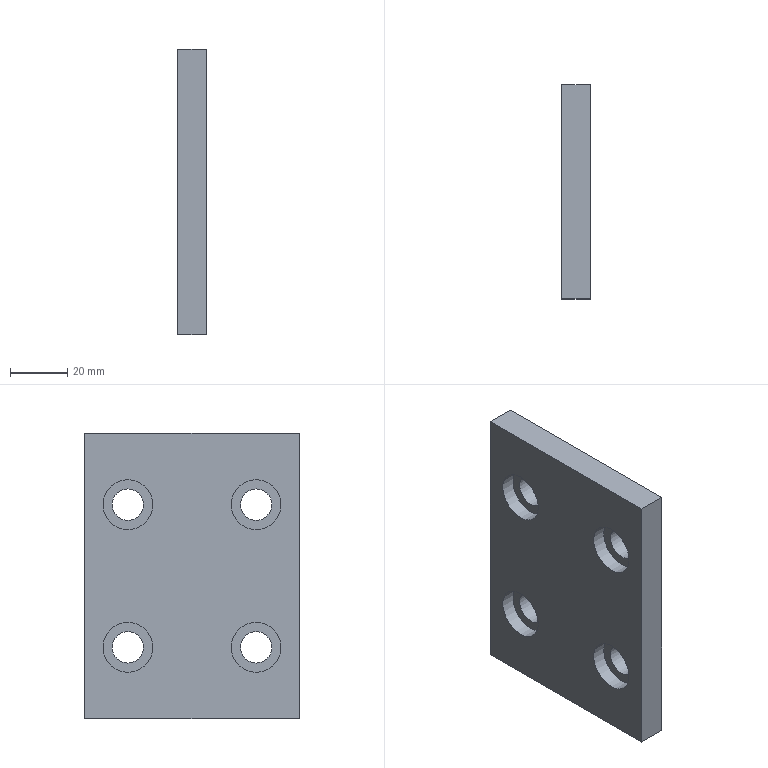Part | NX | features solid 2 | 1 solid | 18 faces | box 10 x 75 x 100 mm | volume 68289 mm3 | plane 10 | cylinder 8 | commonest cylinder face diameters 11 x4 17.5 x4
STEP:
#1=CARTESIAN_POINT('',(-885.,-217.5,218.75));
#2=VERTEX_POINT('',#1);
#3=CARTESIAN_POINT('',(-885.,-217.5,210.));
#4=DIRECTION('',(-1.,0.,0.));
#5=DIRECTION('',(0.,0.,1.));
#6=AXIS2_PLACEMENT_3D('',#3,#4,#5);
#7=CIRCLE('',#6,8.75);
#8=EDGE_CURVE('',#2,#2,#7,.T.);
#9=ORIENTED_EDGE('',*,*,#8,.T.);
#10=EDGE_LOOP('',(#9));
#11=FACE_BOUND('',#10,.T.);
#12=CARTESIAN_POINT('',(-885.,-217.5,204.5));
#13=VERTEX_POINT('',#12);
#14=CARTESIAN_POINT('',(-885.,-217.5,210.));
#15=DIRECTION('',(1.,0.,0.));
#16=DIRECTION('',(0.,0.,-1.));
#17=AXIS2_PLACEMENT_3D('',#14,#15,#16);
#18=CIRCLE('',#17,5.5);
#19=EDGE_CURVE('',#13,#13,#18,.F.);
#20=ORIENTED_EDGE('',*,*,#19,.F.);
#21=EDGE_LOOP('',(#20));
#22=FACE_BOUND('',#21,.T.);
#23=CARTESIAN_POINT('',(-885.,-217.5,210.));
#24=DIRECTION('',(1.,0.,0.));
#25=DIRECTION('',(0.,0.,-1.));
#26=AXIS2_PLACEMENT_3D('',#23,#24,#25);
#27=PLANE('',#26);
#28=ADVANCED_FACE('',(#11,#22),#27,.F.);
#29=CARTESIAN_POINT('',(-885.,-217.5,168.75));
#30=VERTEX_POINT('',#29);
#31=CARTESIAN_POINT('',(-885.,-217.5,160.));
#32=DIRECTION('',(-1.,0.,0.));
#33=DIRECTION('',(0.,0.,1.));
#34=AXIS2_PLACEMENT_3D('',#31,#32,#33);
#35=CIRCLE('',#34,8.75);
#36=EDGE_CURVE('',#30,#30,#35,.T.);
#37=ORIENTED_EDGE('',*,*,#36,.T.);
#38=EDGE_LOOP('',(#37));
#39=FACE_BOUND('',#38,.T.);
#40=CARTESIAN_POINT('',(-885.,-217.5,154.5));
#41=VERTEX_POINT('',#40);
#42=CARTESIAN_POINT('',(-885.,-217.5,160.));
#43=DIRECTION('',(1.,0.,0.));
#44=DIRECTION('',(0.,0.,-1.));
#45=AXIS2_PLACEMENT_3D('',#42,#43,#44);
#46=CIRCLE('',#45,5.5);
#47=EDGE_CURVE('',#41,#41,#46,.F.);
#48=ORIENTED_EDGE('',*,*,#47,.F.);
#49=EDGE_LOOP('',(#48));
#50=FACE_BOUND('',#49,.T.);
#51=CARTESIAN_POINT('',(-885.,-217.5,160.));
#52=DIRECTION('',(1.,0.,0.));
#53=DIRECTION('',(0.,0.,-1.));
#54=AXIS2_PLACEMENT_3D('',#51,#52,#53);
#55=PLANE('',#54);
#56=ADVANCED_FACE('',(#39,#50),#55,.F.);
#57=CARTESIAN_POINT('',(-890.,-217.5,218.75));
#58=VERTEX_POINT('',#57);
#59=CARTESIAN_POINT('',(-890.,-217.5,210.));
#60=DIRECTION('',(-1.,0.,0.));
#61=DIRECTION('',(0.,0.,1.));
#62=AXIS2_PLACEMENT_3D('',#59,#60,#61);
#63=CIRCLE('',#62,8.75);
#64=EDGE_CURVE('',#58,#58,#63,.F.);
#65=ORIENTED_EDGE('',*,*,#64,.F.);
#66=EDGE_LOOP('',(#65));
#67=FACE_BOUND('',#66,.T.);
#68=ORIENTED_EDGE('',*,*,#8,.F.);
#69=EDGE_LOOP('',(#68));
#70=FACE_BOUND('',#69,.T.);
#71=CARTESIAN_POINT('',(-885.,-217.5,210.));
#72=DIRECTION('',(-1.,0.,0.));
#73=DIRECTION('',(0.,0.,1.));
#74=AXIS2_PLACEMENT_3D('',#71,#72,#73);
#75=CYLINDRICAL_SURFACE('',#74,8.75);
#76=ADVANCED_FACE('',(#67,#70),#75,.F.);
#77=CARTESIAN_POINT('',(-890.,-217.5,168.75));
#78=VERTEX_POINT('',#77);
#79=CARTESIAN_POINT('',(-890.,-217.5,160.));
#80=DIRECTION('',(-1.,0.,0.));
#81=DIRECTION('',(0.,0.,1.));
#82=AXIS2_PLACEMENT_3D('',#79,#80,#81);
#83=CIRCLE('',#82,8.75);
#84=EDGE_CURVE('',#78,#78,#83,.F.);
#85=ORIENTED_EDGE('',*,*,#84,.F.);
#86=EDGE_LOOP('',(#85));
#87=FACE_BOUND('',#86,.T.);
#88=ORIENTED_EDGE('',*,*,#36,.F.);
#89=EDGE_LOOP('',(#88));
#90=FACE_BOUND('',#89,.T.);
#91=CARTESIAN_POINT('',(-885.,-217.5,160.));
#92=DIRECTION('',(-1.,0.,0.));
#93=DIRECTION('',(0.,0.,1.));
#94=AXIS2_PLACEMENT_3D('',#91,#92,#93);
#95=CYLINDRICAL_SURFACE('',#94,8.75);
#96=ADVANCED_FACE('',(#87,#90),#95,.F.);
#97=CARTESIAN_POINT('',(-890.,-202.5,135.));
#98=VERTEX_POINT('',#97);
#99=CARTESIAN_POINT('',(-890.,-202.5,235.));
#100=VERTEX_POINT('',#99);
#101=CARTESIAN_POINT('',(-890.,-202.5,135.));
#102=DIRECTION('',(0.,0.,1.));
#103=VECTOR('',#102,1000.);
#104=LINE('',#101,#103);
#105=EDGE_CURVE('',#98,#100,#104,.T.);
#106=ORIENTED_EDGE('',*,*,#105,.T.);
#107=CARTESIAN_POINT('',(-880.,-202.5,235.));
#108=VERTEX_POINT('',#107);
#109=CARTESIAN_POINT('',(-890.,-202.5,235.));
#110=DIRECTION('',(1.,0.,0.));
#111=VECTOR('',#110,1000.);
#112=LINE('',#109,#111);
#113=EDGE_CURVE('',#100,#108,#112,.T.);
#114=ORIENTED_EDGE('',*,*,#113,.T.);
#115=CARTESIAN_POINT('',(-880.,-202.5,135.));
#116=VERTEX_POINT('',#115);
#117=CARTESIAN_POINT('',(-880.,-202.5,135.));
#118=DIRECTION('',(0.,0.,1.));
#119=VECTOR('',#118,1000.);
#120=LINE('',#117,#119);
#121=EDGE_CURVE('',#116,#108,#120,.T.);
#122=ORIENTED_EDGE('',*,*,#121,.F.);
#123=CARTESIAN_POINT('',(-890.,-202.5,135.));
#124=DIRECTION('',(-1.,0.,0.));
#125=VECTOR('',#124,1000.);
#126=LINE('',#123,#125);
#127=EDGE_CURVE('',#116,#98,#126,.T.);
#128=ORIENTED_EDGE('',*,*,#127,.T.);
#129=EDGE_LOOP('',(#106,#114,#122,#128));
#130=FACE_BOUND('',#129,.T.);
#131=CARTESIAN_POINT('',(-890.,-202.5,135.));
#132=DIRECTION('',(0.,1.,0.));
#133=DIRECTION('',(0.,0.,1.));
#134=AXIS2_PLACEMENT_3D('',#131,#132,#133);
#135=PLANE('',#134);
#136=ADVANCED_FACE('',(#130),#135,.T.);
#137=ORIENTED_EDGE('',*,*,#19,.T.);
#138=EDGE_LOOP('',(#137));
#139=FACE_BOUND('',#138,.T.);
#140=CARTESIAN_POINT('',(-880.,-217.5,215.5));
#141=VERTEX_POINT('',#140);
#142=CARTESIAN_POINT('',(-880.,-217.5,210.));
#143=DIRECTION('',(-1.,0.,0.));
#144=DIRECTION('',(0.,0.,1.));
#145=AXIS2_PLACEMENT_3D('',#142,#143,#144);
#146=CIRCLE('',#145,5.5);
#147=EDGE_CURVE('',#141,#141,#146,.T.);
#148=ORIENTED_EDGE('',*,*,#147,.F.);
#149=EDGE_LOOP('',(#148));
#150=FACE_BOUND('',#149,.T.);
#151=CARTESIAN_POINT('',(-880.,-217.5,210.));
#152=DIRECTION('',(-1.,0.,0.));
#153=DIRECTION('',(0.,0.,1.));
#154=AXIS2_PLACEMENT_3D('',#151,#152,#153);
#155=CYLINDRICAL_SURFACE('',#154,5.5);
#156=ADVANCED_FACE('',(#139,#150),#155,.F.);
#157=ORIENTED_EDGE('',*,*,#47,.T.);
#158=EDGE_LOOP('',(#157));
#159=FACE_BOUND('',#158,.T.);
#160=CARTESIAN_POINT('',(-880.,-217.5,165.5));
#161=VERTEX_POINT('',#160);
#162=CARTESIAN_POINT('',(-880.,-217.5,160.));
#163=DIRECTION('',(-1.,0.,0.));
#164=DIRECTION('',(0.,0.,1.));
#165=AXIS2_PLACEMENT_3D('',#162,#163,#164);
#166=CIRCLE('',#165,5.5);
#167=EDGE_CURVE('',#161,#161,#166,.T.);
#168=ORIENTED_EDGE('',*,*,#167,.F.);
#169=EDGE_LOOP('',(#168));
#170=FACE_BOUND('',#169,.T.);
#171=CARTESIAN_POINT('',(-880.,-217.5,160.));
#172=DIRECTION('',(-1.,0.,0.));
#173=DIRECTION('',(0.,0.,1.));
#174=AXIS2_PLACEMENT_3D('',#171,#172,#173);
#175=CYLINDRICAL_SURFACE('',#174,5.5);
#176=ADVANCED_FACE('',(#159,#170),#175,.F.);
#177=ORIENTED_EDGE('',*,*,#167,.T.);
#178=EDGE_LOOP('',(#177));
#179=FACE_BOUND('',#178,.T.);
#180=ORIENTED_EDGE('',*,*,#147,.T.);
#181=EDGE_LOOP('',(#180));
#182=FACE_BOUND('',#181,.T.);
#183=CARTESIAN_POINT('',(-880.,-277.5,235.));
#184=VERTEX_POINT('',#183);
#185=CARTESIAN_POINT('',(-880.,-242.5,235.));
#186=DIRECTION('',(0.,-1.,0.));
#187=VECTOR('',#186,1000.);
#188=LINE('',#185,#187);
#189=EDGE_CURVE('',#108,#184,#188,.T.);
#190=ORIENTED_EDGE('',*,*,#189,.T.);
#191=CARTESIAN_POINT('',(-880.,-277.5,135.));
#192=VERTEX_POINT('',#191);
#193=CARTESIAN_POINT('',(-880.,-277.5,135.));
#194=DIRECTION('',(0.,0.,1.));
#195=VECTOR('',#194,1000.);
#196=LINE('',#193,#195);
#197=EDGE_CURVE('',#192,#184,#196,.T.);
#198=ORIENTED_EDGE('',*,*,#197,.F.);
#199=CARTESIAN_POINT('',(-880.,-242.5,135.));
#200=DIRECTION('',(0.,1.,0.));
#201=VECTOR('',#200,1000.);
#202=LINE('',#199,#201);
#203=EDGE_CURVE('',#192,#116,#202,.T.);
#204=ORIENTED_EDGE('',*,*,#203,.T.);
#205=ORIENTED_EDGE('',*,*,#121,.T.);
#206=EDGE_LOOP('',(#190,#198,#204,#205));
#207=FACE_BOUND('',#206,.T.);
#208=CARTESIAN_POINT('',(-880.,-262.5,165.5));
#209=VERTEX_POINT('',#208);
#210=CARTESIAN_POINT('',(-880.,-262.5,160.));
#211=DIRECTION('',(-1.,0.,0.));
#212=DIRECTION('',(0.,0.,1.));
#213=AXIS2_PLACEMENT_3D('',#210,#211,#212);
#214=CIRCLE('',#213,5.5);
#215=EDGE_CURVE('',#209,#209,#214,.T.);
#216=ORIENTED_EDGE('',*,*,#215,.T.);
#217=EDGE_LOOP('',(#216));
#218=FACE_BOUND('',#217,.T.);
#219=CARTESIAN_POINT('',(-880.,-262.5,215.5));
#220=VERTEX_POINT('',#219);
#221=CARTESIAN_POINT('',(-880.,-262.5,210.));
#222=DIRECTION('',(-1.,0.,0.));
#223=DIRECTION('',(0.,0.,1.));
#224=AXIS2_PLACEMENT_3D('',#221,#222,#223);
#225=CIRCLE('',#224,5.5);
#226=EDGE_CURVE('',#220,#220,#225,.T.);
#227=ORIENTED_EDGE('',*,*,#226,.T.);
#228=EDGE_LOOP('',(#227));
#229=FACE_BOUND('',#228,.T.);
#230=CARTESIAN_POINT('',(-880.,-242.5,135.));
#231=DIRECTION('',(1.,0.,0.));
#232=DIRECTION('',(0.,0.,-1.));
#233=AXIS2_PLACEMENT_3D('',#230,#231,#232);
#234=PLANE('',#233);
#235=ADVANCED_FACE('',(#179,#182,#207,#218,#229),#234,.T.);
#236=ORIENTED_EDGE('',*,*,#203,.F.);
#237=CARTESIAN_POINT('',(-890.,-277.5,135.));
#238=VERTEX_POINT('',#237);
#239=CARTESIAN_POINT('',(-890.,-277.5,135.));
#240=DIRECTION('',(1.,0.,0.));
#241=VECTOR('',#240,1000.);
#242=LINE('',#239,#241);
#243=EDGE_CURVE('',#238,#192,#242,.T.);
#244=ORIENTED_EDGE('',*,*,#243,.F.);
#245=CARTESIAN_POINT('',(-890.,-242.5,135.));
#246=DIRECTION('',(0.,-1.,0.));
#247=VECTOR('',#246,1000.);
#248=LINE('',#245,#247);
#249=EDGE_CURVE('',#98,#238,#248,.T.);
#250=ORIENTED_EDGE('',*,*,#249,.F.);
#251=ORIENTED_EDGE('',*,*,#127,.F.);
#252=EDGE_LOOP('',(#236,#244,#250,#251));
#253=FACE_BOUND('',#252,.T.);
#254=CARTESIAN_POINT('',(-890.,-242.5,135.));
#255=DIRECTION('',(0.,0.,-1.));
#256=DIRECTION('',(-1.,0.,0.));
#257=AXIS2_PLACEMENT_3D('',#254,#255,#256);
#258=PLANE('',#257);
#259=ADVANCED_FACE('',(#253),#258,.T.);
#260=ORIENTED_EDGE('',*,*,#84,.T.);
#261=EDGE_LOOP('',(#260));
#262=FACE_BOUND('',#261,.T.);
#263=ORIENTED_EDGE('',*,*,#64,.T.);
#264=EDGE_LOOP('',(#263));
#265=FACE_BOUND('',#264,.T.);
#266=ORIENTED_EDGE('',*,*,#249,.T.);
#267=CARTESIAN_POINT('',(-890.,-277.5,235.));
#268=VERTEX_POINT('',#267);
#269=CARTESIAN_POINT('',(-890.,-277.5,135.));
#270=DIRECTION('',(0.,0.,1.));
#271=VECTOR('',#270,1000.);
#272=LINE('',#269,#271);
#273=EDGE_CURVE('',#238,#268,#272,.T.);
#274=ORIENTED_EDGE('',*,*,#273,.T.);
#275=CARTESIAN_POINT('',(-890.,-242.5,235.));
#276=DIRECTION('',(0.,1.,0.));
#277=VECTOR('',#276,1000.);
#278=LINE('',#275,#277);
#279=EDGE_CURVE('',#268,#100,#278,.T.);
#280=ORIENTED_EDGE('',*,*,#279,.T.);
#281=ORIENTED_EDGE('',*,*,#105,.F.);
#282=EDGE_LOOP('',(#266,#274,#280,#281));
#283=FACE_BOUND('',#282,.T.);
#284=CARTESIAN_POINT('',(-890.,-262.5,168.75));
#285=VERTEX_POINT('',#284);
#286=CARTESIAN_POINT('',(-890.,-262.5,160.));
#287=DIRECTION('',(-1.,0.,0.));
#288=DIRECTION('',(0.,0.,1.));
#289=AXIS2_PLACEMENT_3D('',#286,#287,#288);
#290=CIRCLE('',#289,8.75);
#291=EDGE_CURVE('',#285,#285,#290,.F.);
#292=ORIENTED_EDGE('',*,*,#291,.T.);
#293=EDGE_LOOP('',(#292));
#294=FACE_BOUND('',#293,.T.);
#295=CARTESIAN_POINT('',(-890.,-262.5,218.75));
#296=VERTEX_POINT('',#295);
#297=CARTESIAN_POINT('',(-890.,-262.5,210.));
#298=DIRECTION('',(-1.,0.,0.));
#299=DIRECTION('',(0.,0.,1.));
#300=AXIS2_PLACEMENT_3D('',#297,#298,#299);
#301=CIRCLE('',#300,8.75);
#302=EDGE_CURVE('',#296,#296,#301,.F.);
#303=ORIENTED_EDGE('',*,*,#302,.T.);
#304=EDGE_LOOP('',(#303));
#305=FACE_BOUND('',#304,.T.);
#306=CARTESIAN_POINT('',(-890.,-242.5,135.));
#307=DIRECTION('',(-1.,0.,0.));
#308=DIRECTION('',(0.,0.,1.));
#309=AXIS2_PLACEMENT_3D('',#306,#307,#308);
#310=PLANE('',#309);
#311=ADVANCED_FACE('',(#262,#265,#283,#294,#305),#310,.T.);
#312=ORIENTED_EDGE('',*,*,#279,.F.);
#313=CARTESIAN_POINT('',(-890.,-277.5,235.));
#314=DIRECTION('',(-1.,0.,0.));
#315=VECTOR('',#314,1000.);
#316=LINE('',#313,#315);
#317=EDGE_CURVE('',#184,#268,#316,.T.);
#318=ORIENTED_EDGE('',*,*,#317,.F.);
#319=ORIENTED_EDGE('',*,*,#189,.F.);
#320=ORIENTED_EDGE('',*,*,#113,.F.);
#321=EDGE_LOOP('',(#312,#318,#319,#320));
#322=FACE_BOUND('',#321,.T.);
#323=CARTESIAN_POINT('',(-890.,-242.5,235.));
#324=DIRECTION('',(0.,0.,1.));
#325=DIRECTION('',(1.,0.,0.));
#326=AXIS2_PLACEMENT_3D('',#323,#324,#325);
#327=PLANE('',#326);
#328=ADVANCED_FACE('',(#322),#327,.T.);
#329=CARTESIAN_POINT('',(-885.,-262.5,204.5));
#330=VERTEX_POINT('',#329);
#331=CARTESIAN_POINT('',(-885.,-262.5,210.));
#332=DIRECTION('',(1.,0.,0.));
#333=DIRECTION('',(0.,0.,-1.));
#334=AXIS2_PLACEMENT_3D('',#331,#332,#333);
#335=CIRCLE('',#334,5.5);
#336=EDGE_CURVE('',#330,#330,#335,.F.);
#337=ORIENTED_EDGE('',*,*,#336,.T.);
#338=EDGE_LOOP('',(#337));
#339=FACE_BOUND('',#338,.T.);
#340=ORIENTED_EDGE('',*,*,#226,.F.);
#341=EDGE_LOOP('',(#340));
#342=FACE_BOUND('',#341,.T.);
#343=CARTESIAN_POINT('',(-880.,-262.5,210.));
#344=DIRECTION('',(-1.,0.,0.));
#345=DIRECTION('',(0.,0.,1.));
#346=AXIS2_PLACEMENT_3D('',#343,#344,#345);
#347=CYLINDRICAL_SURFACE('',#346,5.5);
#348=ADVANCED_FACE('',(#339,#342),#347,.F.);
#349=CARTESIAN_POINT('',(-885.,-262.5,218.75));
#350=VERTEX_POINT('',#349);
#351=CARTESIAN_POINT('',(-885.,-262.5,210.));
#352=DIRECTION('',(-1.,0.,0.));
#353=DIRECTION('',(0.,0.,1.));
#354=AXIS2_PLACEMENT_3D('',#351,#352,#353);
#355=CIRCLE('',#354,8.75);
#356=EDGE_CURVE('',#350,#350,#355,.T.);
#357=ORIENTED_EDGE('',*,*,#356,.T.);
#358=EDGE_LOOP('',(#357));
#359=FACE_BOUND('',#358,.T.);
#360=ORIENTED_EDGE('',*,*,#336,.F.);
#361=EDGE_LOOP('',(#360));
#362=FACE_BOUND('',#361,.T.);
#363=CARTESIAN_POINT('',(-885.,-262.5,210.));
#364=DIRECTION('',(1.,0.,0.));
#365=DIRECTION('',(0.,0.,-1.));
#366=AXIS2_PLACEMENT_3D('',#363,#364,#365);
#367=PLANE('',#366);
#368=ADVANCED_FACE('',(#359,#362),#367,.F.);
#369=ORIENTED_EDGE('',*,*,#302,.F.);
#370=EDGE_LOOP('',(#369));
#371=FACE_BOUND('',#370,.T.);
#372=ORIENTED_EDGE('',*,*,#356,.F.);
#373=EDGE_LOOP('',(#372));
#374=FACE_BOUND('',#373,.T.);
#375=CARTESIAN_POINT('',(-885.,-262.5,210.));
#376=DIRECTION('',(-1.,0.,0.));
#377=DIRECTION('',(0.,0.,1.));
#378=AXIS2_PLACEMENT_3D('',#375,#376,#377);
#379=CYLINDRICAL_SURFACE('',#378,8.75);
#380=ADVANCED_FACE('',(#371,#374),#379,.F.);
#381=CARTESIAN_POINT('',(-885.,-262.5,154.5));
#382=VERTEX_POINT('',#381);
#383=CARTESIAN_POINT('',(-885.,-262.5,160.));
#384=DIRECTION('',(1.,0.,0.));
#385=DIRECTION('',(0.,0.,-1.));
#386=AXIS2_PLACEMENT_3D('',#383,#384,#385);
#387=CIRCLE('',#386,5.5);
#388=EDGE_CURVE('',#382,#382,#387,.F.);
#389=ORIENTED_EDGE('',*,*,#388,.T.);
#390=EDGE_LOOP('',(#389));
#391=FACE_BOUND('',#390,.T.);
#392=ORIENTED_EDGE('',*,*,#215,.F.);
#393=EDGE_LOOP('',(#392));
#394=FACE_BOUND('',#393,.T.);
#395=CARTESIAN_POINT('',(-880.,-262.5,160.));
#396=DIRECTION('',(-1.,0.,0.));
#397=DIRECTION('',(0.,0.,1.));
#398=AXIS2_PLACEMENT_3D('',#395,#396,#397);
#399=CYLINDRICAL_SURFACE('',#398,5.5);
#400=ADVANCED_FACE('',(#391,#394),#399,.F.);
#401=CARTESIAN_POINT('',(-885.,-262.5,168.75));
#402=VERTEX_POINT('',#401);
#403=CARTESIAN_POINT('',(-885.,-262.5,160.));
#404=DIRECTION('',(-1.,0.,0.));
#405=DIRECTION('',(0.,0.,1.));
#406=AXIS2_PLACEMENT_3D('',#403,#404,#405);
#407=CIRCLE('',#406,8.75);
#408=EDGE_CURVE('',#402,#402,#407,.T.);
#409=ORIENTED_EDGE('',*,*,#408,.T.);
#410=EDGE_LOOP('',(#409));
#411=FACE_BOUND('',#410,.T.);
#412=ORIENTED_EDGE('',*,*,#388,.F.);
#413=EDGE_LOOP('',(#412));
#414=FACE_BOUND('',#413,.T.);
#415=CARTESIAN_POINT('',(-885.,-262.5,160.));
#416=DIRECTION('',(1.,0.,0.));
#417=DIRECTION('',(0.,0.,-1.));
#418=AXIS2_PLACEMENT_3D('',#415,#416,#417);
#419=PLANE('',#418);
#420=ADVANCED_FACE('',(#411,#414),#419,.F.);
#421=ORIENTED_EDGE('',*,*,#291,.F.);
#422=EDGE_LOOP('',(#421));
#423=FACE_BOUND('',#422,.T.);
#424=ORIENTED_EDGE('',*,*,#408,.F.);
#425=EDGE_LOOP('',(#424));
#426=FACE_BOUND('',#425,.T.);
#427=CARTESIAN_POINT('',(-885.,-262.5,160.));
#428=DIRECTION('',(-1.,0.,0.));
#429=DIRECTION('',(0.,0.,1.));
#430=AXIS2_PLACEMENT_3D('',#427,#428,#429);
#431=CYLINDRICAL_SURFACE('',#430,8.75);
#432=ADVANCED_FACE('',(#423,#426),#431,.F.);
#433=ORIENTED_EDGE('',*,*,#197,.T.);
#434=ORIENTED_EDGE('',*,*,#317,.T.);
#435=ORIENTED_EDGE('',*,*,#273,.F.);
#436=ORIENTED_EDGE('',*,*,#243,.T.);
#437=EDGE_LOOP('',(#433,#434,#435,#436));
#438=FACE_BOUND('',#437,.T.);
#439=CARTESIAN_POINT('',(-890.,-277.5,135.));
#440=DIRECTION('',(0.,-1.,0.));
#441=DIRECTION('',(0.,0.,-1.));
#442=AXIS2_PLACEMENT_3D('',#439,#440,#441);
#443=PLANE('',#442);
#444=ADVANCED_FACE('',(#438),#443,.T.);
#445=CLOSED_SHELL('',(#28,#56,#76,#96,#136,#156,#176,#235,#259,#311,#328,#348,#368,#380,#400,#420,#432,#444));
#446=MANIFOLD_SOLID_BREP('',#445);
#447=(LENGTH_UNIT()NAMED_UNIT(*)SI_UNIT(.MILLI.,.METRE.));
#448=UNCERTAINTY_MEASURE_WITH_UNIT(LENGTH_MEASURE(0.00001),#447,'','');
#449=(NAMED_UNIT(*)PLANE_ANGLE_UNIT()SI_UNIT($,.RADIAN.));
#450=(NAMED_UNIT(*)SI_UNIT($,.STERADIAN.)SOLID_ANGLE_UNIT());
#451=(GEOMETRIC_REPRESENTATION_CONTEXT(3)GLOBAL_UNCERTAINTY_ASSIGNED_CONTEXT((#448))GLOBAL_UNIT_ASSIGNED_CONTEXT((#447,#449,#450))REPRESENTATION_CONTEXT('',''));
#452=ADVANCED_BREP_SHAPE_REPRESENTATION('',(#446),#451);